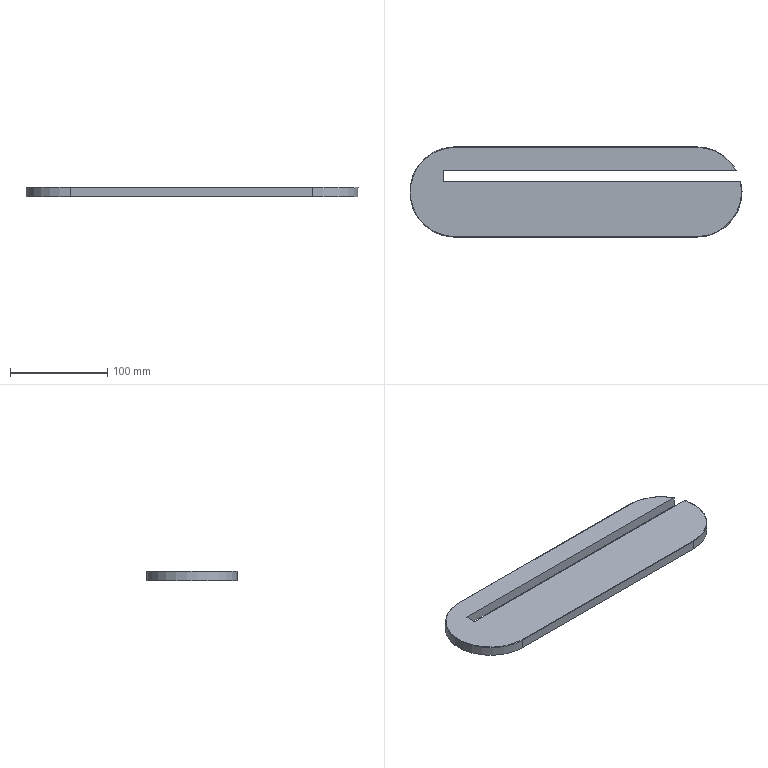Part | STEP file | DEWALT-DWE7492-B22 | 1 solid | 15 faces | box 342.3 x 93 x 10 mm | volume 265013 mm3 | plane 7 | cylinder 5 | torus 3 | commonest cylinder face diameters 93 x3 1 x2
STEP:
#1=CARTESIAN_POINT('',(0.,0.,0.));
#2=DIRECTION('',(0.,0.,1.));
#3=DIRECTION('',(1.,0.,0.));
#4=AXIS2_PLACEMENT_3D('',#1,#2,#3);
#5=CARTESIAN_POINT('',(-86.5,-1.8,30.));
#6=VERTEX_POINT('',#5);
#7=CARTESIAN_POINT('',(220.004,-1.8,30.));
#8=VERTEX_POINT('',#7);
#9=CARTESIAN_POINT('',(66.752,-1.8,30.));
#10=DIRECTION('',(1.,0.,0.));
#11=VECTOR('',#10,1.);
#12=LINE('',#9,#11);
#13=CARTESIAN_POINT('',(-86.51,-1.8,40.01));
#14=DIRECTION('',(0.,1.,0.));
#15=DIRECTION('',(1.,0.,0.));
#16=AXIS2_PLACEMENT_3D('',#13,#14,#15);
#17=PLANE('',#16);
#18=CARTESIAN_POINT('',(153.262,10.01));
#19=DIRECTION('',(1.,0.));
#20=VECTOR('',#19,1.);
#21=LINE('',#18,#20);
#22=(GEOMETRIC_REPRESENTATION_CONTEXT(2)PARAMETRIC_REPRESENTATION_CONTEXT()REPRESENTATION_CONTEXT('',''));
#23=DEFINITIONAL_REPRESENTATION('',(#21),#22);
#24=PCURVE('',#17,#23);
#25=CARTESIAN_POINT('',(-121.01,33.81,30.));
#26=DIRECTION('',(0.,0.,-1.));
#27=DIRECTION('',(1.,0.,0.));
#28=AXIS2_PLACEMENT_3D('',#25,#26,#27);
#29=PLANE('',#28);
#30=CARTESIAN_POINT('',(187.762,35.61));
#31=DIRECTION('',(1.,0.));
#32=VECTOR('',#31,1.);
#33=LINE('',#30,#32);
#34=(GEOMETRIC_REPRESENTATION_CONTEXT(2)PARAMETRIC_REPRESENTATION_CONTEXT()REPRESENTATION_CONTEXT('',''));
#35=DEFINITIONAL_REPRESENTATION('',(#33),#34);
#36=PCURVE('',#29,#35);
#37=SURFACE_CURVE('',#12,(#24,#36),.PCURVE_S1.);
#38=EDGE_CURVE('',#6,#8,#37,.T.);
#39=ORIENTED_EDGE('',*,*,#38,.F.);
#40=CARTESIAN_POINT('',(-86.5,-1.8,40.));
#41=VERTEX_POINT('',#40);
#42=CARTESIAN_POINT('',(-86.5,-1.8,35.));
#43=DIRECTION('',(0.,0.,-1.));
#44=VECTOR('',#43,1.);
#45=LINE('',#42,#44);
#46=CARTESIAN_POINT('',(0.01,5.01));
#47=DIRECTION('',(0.,1.));
#48=VECTOR('',#47,1.);
#49=LINE('',#46,#48);
#50=(GEOMETRIC_REPRESENTATION_CONTEXT(2)PARAMETRIC_REPRESENTATION_CONTEXT()REPRESENTATION_CONTEXT('',''));
#51=DEFINITIONAL_REPRESENTATION('',(#49),#50);
#52=PCURVE('',#17,#51);
#53=CARTESIAN_POINT('',(-86.5,9.61,40.01));
#54=DIRECTION('',(1.,0.,0.));
#55=DIRECTION('',(0.,-1.,0.));
#56=AXIS2_PLACEMENT_3D('',#53,#54,#55);
#57=PLANE('',#56);
#58=CARTESIAN_POINT('',(11.41,5.01));
#59=DIRECTION('',(0.,1.));
#60=VECTOR('',#59,1.);
#61=LINE('',#58,#60);
#62=(GEOMETRIC_REPRESENTATION_CONTEXT(2)PARAMETRIC_REPRESENTATION_CONTEXT()REPRESENTATION_CONTEXT('',''));
#63=DEFINITIONAL_REPRESENTATION('',(#61),#62);
#64=PCURVE('',#57,#63);
#65=SURFACE_CURVE('',#45,(#52,#64),.PCURVE_S1.);
#66=EDGE_CURVE('',#41,#6,#65,.T.);
#67=ORIENTED_EDGE('',*,*,#66,.F.);
#68=CARTESIAN_POINT('',(219.49,-1.8,40.));
#69=VERTEX_POINT('',#68);
#70=CARTESIAN_POINT('',(66.495,-1.8,40.));
#71=DIRECTION('',(-1.,0.,0.));
#72=VECTOR('',#71,1.);
#73=LINE('',#70,#72);
#74=CARTESIAN_POINT('',(153.005,0.01));
#75=DIRECTION('',(-1.,0.));
#76=VECTOR('',#75,1.);
#77=LINE('',#74,#76);
#78=(GEOMETRIC_REPRESENTATION_CONTEXT(2)PARAMETRIC_REPRESENTATION_CONTEXT()REPRESENTATION_CONTEXT('',''));
#79=DEFINITIONAL_REPRESENTATION('',(#77),#78);
#80=PCURVE('',#17,#79);
#81=CARTESIAN_POINT('',(224.799,33.31,40.));
#82=DIRECTION('',(0.,0.,1.));
#83=DIRECTION('',(-1.,0.,0.));
#84=AXIS2_PLACEMENT_3D('',#81,#82,#83);
#85=PLANE('',#84);
#86=CARTESIAN_POINT('',(158.304,35.11));
#87=DIRECTION('',(1.,0.));
#88=VECTOR('',#87,1.);
#89=LINE('',#86,#88);
#90=(GEOMETRIC_REPRESENTATION_CONTEXT(2)PARAMETRIC_REPRESENTATION_CONTEXT()REPRESENTATION_CONTEXT('',''));
#91=DEFINITIONAL_REPRESENTATION('',(#89),#90);
#92=PCURVE('',#85,#91);
#93=SURFACE_CURVE('',#73,(#80,#92),.PCURVE_S1.);
#94=EDGE_CURVE('',#69,#41,#93,.T.);
#95=ORIENTED_EDGE('',*,*,#94,.F.);
#96=CARTESIAN_POINT('',(220.004,-1.8,39.5));
#97=VERTEX_POINT('',#96);
#98=CARTESIAN_POINT('',(220.004,-1.8,39.5));
#99=CARTESIAN_POINT('',(220.004,-1.8,39.768));
#100=CARTESIAN_POINT('',(219.758,-1.8,40.));
#101=CARTESIAN_POINT('',(219.49,-1.8,40.));
#102=B_SPLINE_CURVE_WITH_KNOTS('',3,(#98,#99,#100,#101),.UNSPECIFIED.,.F.,.F.,(4,4),(0.,0.0007925),.PIECEWISE_BEZIER_KNOTS.);
#103=CARTESIAN_POINT('',(306.514,0.51));
#104=CARTESIAN_POINT('',(306.514,0.242));
#105=CARTESIAN_POINT('',(306.268,0.01));
#106=CARTESIAN_POINT('',(306.,0.01));
#107=B_SPLINE_CURVE_WITH_KNOTS('',3,(#103,#104,#105,#106),.UNSPECIFIED.,.F.,.F.,(4,4),(0.,0.0007925),.PIECEWISE_BEZIER_KNOTS.);
#108=(GEOMETRIC_REPRESENTATION_CONTEXT(2)PARAMETRIC_REPRESENTATION_CONTEXT()REPRESENTATION_CONTEXT('',''));
#109=DEFINITIONAL_REPRESENTATION('',(#107),#108);
#110=PCURVE('',#17,#109);
#111=CARTESIAN_POINT('',(174.8,-12.7,39.5));
#112=DIRECTION('',(0.,0.,1.));
#113=DIRECTION('',(0.,-1.,0.));
#114=AXIS2_PLACEMENT_3D('',#111,#112,#113);
#115=TOROIDAL_SURFACE('',#114,46.,0.5);
#116=CARTESIAN_POINT('',(1.807,0.));
#117=CARTESIAN_POINT('',(1.807,0.02436));
#118=CARTESIAN_POINT('',(1.807,0.0728));
#119=CARTESIAN_POINT('',(1.807,0.1448));
#120=CARTESIAN_POINT('',(1.807,0.2165));
#121=CARTESIAN_POINT('',(1.808,0.288));
#122=CARTESIAN_POINT('',(1.808,0.3594));
#123=CARTESIAN_POINT('',(1.808,0.4308));
#124=CARTESIAN_POINT('',(1.808,0.5024));
#125=CARTESIAN_POINT('',(1.808,0.5741));
#126=CARTESIAN_POINT('',(1.808,0.6458));
#127=CARTESIAN_POINT('',(1.808,0.7177));
#128=CARTESIAN_POINT('',(1.808,0.7896));
#129=CARTESIAN_POINT('',(1.808,0.8615));
#130=CARTESIAN_POINT('',(1.808,0.9332));
#131=CARTESIAN_POINT('',(1.809,1.005));
#132=CARTESIAN_POINT('',(1.809,1.076));
#133=CARTESIAN_POINT('',(1.809,1.147));
#134=CARTESIAN_POINT('',(1.809,1.218));
#135=CARTESIAN_POINT('',(1.809,1.289));
#136=CARTESIAN_POINT('',(1.809,1.359));
#137=CARTESIAN_POINT('',(1.81,1.43));
#138=CARTESIAN_POINT('',(1.81,1.5));
#139=CARTESIAN_POINT('',(1.81,1.547));
#140=CARTESIAN_POINT('',(1.81,1.571));
#141=B_SPLINE_CURVE_WITH_KNOTS('',3,(#116,#117,#118,#119,#120,#121,#122,#123,#124,#125,#126,#127,#128,#129,#130,#131,#132,#133,#134,#135,#136,#137,#138,#139,#140),.UNSPECIFIED.,.F.,.F.,(4,1,1,1,1,1,1,1,1,1,1,1,1,1,1,1,1,1,1,1,1,1,4),(0.,0.00003602,0.00007204,0.0001081,0.0001441,0.0001801,0.0002161,0.0002521,0.0002882,0.0003242,0.0003602,0.0003962,0.0004323,0.0004683,0.0005043,0.0005403,0.0005763,0.0006124,0.0006484,0.0006844,0.0007204,0.0007564,0.0007925),.QUASI_UNIFORM_KNOTS.);
#142=(GEOMETRIC_REPRESENTATION_CONTEXT(2)PARAMETRIC_REPRESENTATION_CONTEXT()REPRESENTATION_CONTEXT('',''));
#143=DEFINITIONAL_REPRESENTATION('',(#141),#142);
#144=PCURVE('',#115,#143);
#145=SURFACE_CURVE('',#102,(#110,#144),.PCURVE_S1.);
#146=EDGE_CURVE('',#97,#69,#145,.T.);
#147=ORIENTED_EDGE('',*,*,#146,.F.);
#148=CARTESIAN_POINT('',(220.004,-1.8,34.75));
#149=DIRECTION('',(0.,0.,1.));
#150=VECTOR('',#149,1.);
#151=LINE('',#148,#150);
#152=CARTESIAN_POINT('',(306.514,5.26));
#153=DIRECTION('',(0.,-1.));
#154=VECTOR('',#153,1.);
#155=LINE('',#152,#154);
#156=(GEOMETRIC_REPRESENTATION_CONTEXT(2)PARAMETRIC_REPRESENTATION_CONTEXT()REPRESENTATION_CONTEXT('',''));
#157=DEFINITIONAL_REPRESENTATION('',(#155),#156);
#158=PCURVE('',#17,#157);
#159=CARTESIAN_POINT('',(174.8,-12.7,30.));
#160=DIRECTION('',(0.,0.,1.));
#161=DIRECTION('',(1.,0.,0.));
#162=AXIS2_PLACEMENT_3D('',#159,#160,#161);
#163=CYLINDRICAL_SURFACE('',#162,46.5);
#164=CARTESIAN_POINT('',(6.52,4.75));
#165=DIRECTION('',(0.,1.));
#166=VECTOR('',#165,1.);
#167=LINE('',#164,#166);
#168=(GEOMETRIC_REPRESENTATION_CONTEXT(2)PARAMETRIC_REPRESENTATION_CONTEXT()REPRESENTATION_CONTEXT('',''));
#169=DEFINITIONAL_REPRESENTATION('',(#167),#168);
#170=PCURVE('',#163,#169);
#171=SURFACE_CURVE('',#151,(#158,#170),.PCURVE_S1.);
#172=EDGE_CURVE('',#8,#97,#171,.T.);
#173=ORIENTED_EDGE('',*,*,#172,.F.);
#174=EDGE_LOOP('',(#39,#67,#95,#147,#173));
#175=FACE_BOUND('',#174,.T.);
#176=ADVANCED_FACE('',(#175),#17,.T.);
#177=CARTESIAN_POINT('',(215.604,9.6,30.));
#178=VERTEX_POINT('',#177);
#179=CARTESIAN_POINT('',(-86.5,9.6,30.));
#180=VERTEX_POINT('',#179);
#181=CARTESIAN_POINT('',(64.552,9.6,30.));
#182=DIRECTION('',(-1.,0.,0.));
#183=VECTOR('',#182,1.);
#184=LINE('',#181,#183);
#185=CARTESIAN_POINT('',(215.614,9.6,40.01));
#186=DIRECTION('',(0.,-1.,0.));
#187=DIRECTION('',(-1.,0.,0.));
#188=AXIS2_PLACEMENT_3D('',#185,#186,#187);
#189=PLANE('',#188);
#190=CARTESIAN_POINT('',(151.062,10.01));
#191=DIRECTION('',(1.,0.));
#192=VECTOR('',#191,1.);
#193=LINE('',#190,#192);
#194=(GEOMETRIC_REPRESENTATION_CONTEXT(2)PARAMETRIC_REPRESENTATION_CONTEXT()REPRESENTATION_CONTEXT('',''));
#195=DEFINITIONAL_REPRESENTATION('',(#193),#194);
#196=PCURVE('',#189,#195);
#197=CARTESIAN_POINT('',(185.562,24.21));
#198=DIRECTION('',(-1.,0.));
#199=VECTOR('',#198,1.);
#200=LINE('',#197,#199);
#201=(GEOMETRIC_REPRESENTATION_CONTEXT(2)PARAMETRIC_REPRESENTATION_CONTEXT()REPRESENTATION_CONTEXT('',''));
#202=DEFINITIONAL_REPRESENTATION('',(#200),#201);
#203=PCURVE('',#29,#202);
#204=SURFACE_CURVE('',#184,(#196,#203),.PCURVE_S1.);
#205=EDGE_CURVE('',#178,#180,#204,.T.);
#206=ORIENTED_EDGE('',*,*,#205,.F.);
#207=CARTESIAN_POINT('',(215.604,9.6,39.5));
#208=VERTEX_POINT('',#207);
#209=CARTESIAN_POINT('',(215.604,9.6,34.75));
#210=DIRECTION('',(0.,0.,-1.));
#211=VECTOR('',#210,1.);
#212=LINE('',#209,#211);
#213=CARTESIAN_POINT('',(0.01,5.26));
#214=DIRECTION('',(0.,1.));
#215=VECTOR('',#214,1.);
#216=LINE('',#213,#215);
#217=(GEOMETRIC_REPRESENTATION_CONTEXT(2)PARAMETRIC_REPRESENTATION_CONTEXT()REPRESENTATION_CONTEXT('',''));
#218=DEFINITIONAL_REPRESENTATION('',(#216),#217);
#219=PCURVE('',#189,#218);
#220=CARTESIAN_POINT('',(174.8,-12.7,30.));
#221=DIRECTION('',(0.,0.,1.));
#222=DIRECTION('',(0.,-1.,0.));
#223=AXIS2_PLACEMENT_3D('',#220,#221,#222);
#224=CYLINDRICAL_SURFACE('',#223,46.5);
#225=CARTESIAN_POINT('',(2.071,4.75));
#226=DIRECTION('',(0.,-1.));
#227=VECTOR('',#226,1.);
#228=LINE('',#225,#227);
#229=(GEOMETRIC_REPRESENTATION_CONTEXT(2)PARAMETRIC_REPRESENTATION_CONTEXT()REPRESENTATION_CONTEXT('',''));
#230=DEFINITIONAL_REPRESENTATION('',(#228),#229);
#231=PCURVE('',#224,#230);
#232=SURFACE_CURVE('',#212,(#219,#231),.PCURVE_S1.);
#233=EDGE_CURVE('',#208,#178,#232,.T.);
#234=ORIENTED_EDGE('',*,*,#233,.F.);
#235=CARTESIAN_POINT('',(215.033,9.6,40.));
#236=VERTEX_POINT('',#235);
#237=CARTESIAN_POINT('',(215.033,9.6,40.));
#238=CARTESIAN_POINT('',(215.316,9.6,40.));
#239=CARTESIAN_POINT('',(215.604,9.6,39.784));
#240=CARTESIAN_POINT('',(215.604,9.6,39.5));
#241=B_SPLINE_CURVE_WITH_KNOTS('',3,(#237,#238,#239,#240),.UNSPECIFIED.,.F.,.F.,(4,4),(0.,0.0008376),.PIECEWISE_BEZIER_KNOTS.);
#242=CARTESIAN_POINT('',(0.5807,0.01));
#243=CARTESIAN_POINT('',(0.2976,0.01));
#244=CARTESIAN_POINT('',(0.01,0.2255));
#245=CARTESIAN_POINT('',(0.01,0.51));
#246=B_SPLINE_CURVE_WITH_KNOTS('',3,(#242,#243,#244,#245),.UNSPECIFIED.,.F.,.F.,(4,4),(0.,0.0008376),.PIECEWISE_BEZIER_KNOTS.);
#247=(GEOMETRIC_REPRESENTATION_CONTEXT(2)PARAMETRIC_REPRESENTATION_CONTEXT()REPRESENTATION_CONTEXT('',''));
#248=DEFINITIONAL_REPRESENTATION('',(#246),#247);
#249=PCURVE('',#189,#248);
#250=CARTESIAN_POINT('',(174.8,-12.7,39.5));
#251=DIRECTION('',(0.,0.,1.));
#252=DIRECTION('',(1.,0.,0.));
#253=AXIS2_PLACEMENT_3D('',#250,#251,#252);
#254=TOROIDAL_SURFACE('',#253,46.,0.5);
#255=CARTESIAN_POINT('',(0.5061,1.571));
#256=CARTESIAN_POINT('',(0.506,1.548));
#257=CARTESIAN_POINT('',(0.5057,1.503));
#258=CARTESIAN_POINT('',(0.5053,1.435));
#259=CARTESIAN_POINT('',(0.5049,1.367));
#260=CARTESIAN_POINT('',(0.5045,1.298));
#261=CARTESIAN_POINT('',(0.5041,1.229));
#262=CARTESIAN_POINT('',(0.5037,1.16));
#263=CARTESIAN_POINT('',(0.5034,1.089));
#264=CARTESIAN_POINT('',(0.503,1.019));
#265=CARTESIAN_POINT('',(0.5027,0.9479));
#266=CARTESIAN_POINT('',(0.5023,0.8767));
#267=CARTESIAN_POINT('',(0.502,0.8052));
#268=CARTESIAN_POINT('',(0.5017,0.7336));
#269=CARTESIAN_POINT('',(0.5014,0.6618));
#270=CARTESIAN_POINT('',(0.5012,0.5899));
#271=CARTESIAN_POINT('',(0.501,0.5178));
#272=CARTESIAN_POINT('',(0.5008,0.4456));
#273=CARTESIAN_POINT('',(0.5006,0.3731));
#274=CARTESIAN_POINT('',(0.5004,0.3002));
#275=CARTESIAN_POINT('',(0.5003,0.2267));
#276=CARTESIAN_POINT('',(0.5002,0.1524));
#277=CARTESIAN_POINT('',(0.5002,0.07701));
#278=CARTESIAN_POINT('',(0.5002,0.02586));
#279=CARTESIAN_POINT('',(0.5002,0.));
#280=B_SPLINE_CURVE_WITH_KNOTS('',3,(#255,#256,#257,#258,#259,#260,#261,#262,#263,#264,#265,#266,#267,#268,#269,#270,#271,#272,#273,#274,#275,#276,#277,#278,#279),.UNSPECIFIED.,.F.,.F.,(4,1,1,1,1,1,1,1,1,1,1,1,1,1,1,1,1,1,1,1,1,1,4),(0.,0.00003807,0.00007615,0.0001142,0.0001523,0.0001904,0.0002284,0.0002665,0.0003046,0.0003427,0.0003807,0.0004188,0.0004569,0.000495,0.000533,0.0005711,0.0006092,0.0006473,0.0006853,0.0007234,0.0007615,0.0007996,0.0008376),.QUASI_UNIFORM_KNOTS.);
#281=(GEOMETRIC_REPRESENTATION_CONTEXT(2)PARAMETRIC_REPRESENTATION_CONTEXT()REPRESENTATION_CONTEXT('',''));
#282=DEFINITIONAL_REPRESENTATION('',(#280),#281);
#283=PCURVE('',#254,#282);
#284=SURFACE_CURVE('',#241,(#249,#283),.PCURVE_S1.);
#285=EDGE_CURVE('',#236,#208,#284,.T.);
#286=ORIENTED_EDGE('',*,*,#285,.F.);
#287=CARTESIAN_POINT('',(-86.5,9.6,40.));
#288=VERTEX_POINT('',#287);
#289=CARTESIAN_POINT('',(64.267,9.6,40.));
#290=DIRECTION('',(1.,0.,0.));
#291=VECTOR('',#290,1.);
#292=LINE('',#289,#291);
#293=CARTESIAN_POINT('',(151.347,0.01));
#294=DIRECTION('',(-1.,0.));
#295=VECTOR('',#294,1.);
#296=LINE('',#293,#295);
#297=(GEOMETRIC_REPRESENTATION_CONTEXT(2)PARAMETRIC_REPRESENTATION_CONTEXT()REPRESENTATION_CONTEXT('',''));
#298=DEFINITIONAL_REPRESENTATION('',(#296),#297);
#299=PCURVE('',#189,#298);
#300=CARTESIAN_POINT('',(160.532,23.71));
#301=DIRECTION('',(-1.,0.));
#302=VECTOR('',#301,1.);
#303=LINE('',#300,#302);
#304=(GEOMETRIC_REPRESENTATION_CONTEXT(2)PARAMETRIC_REPRESENTATION_CONTEXT()REPRESENTATION_CONTEXT('',''));
#305=DEFINITIONAL_REPRESENTATION('',(#303),#304);
#306=PCURVE('',#85,#305);
#307=SURFACE_CURVE('',#292,(#299,#306),.PCURVE_S1.);
#308=EDGE_CURVE('',#288,#236,#307,.T.);
#309=ORIENTED_EDGE('',*,*,#308,.F.);
#310=CARTESIAN_POINT('',(-86.5,9.6,35.));
#311=DIRECTION('',(0.,0.,-1.));
#312=VECTOR('',#311,1.);
#313=LINE('',#310,#312);
#314=CARTESIAN_POINT('',(302.114,5.01));
#315=DIRECTION('',(0.,1.));
#316=VECTOR('',#315,1.);
#317=LINE('',#314,#316);
#318=(GEOMETRIC_REPRESENTATION_CONTEXT(2)PARAMETRIC_REPRESENTATION_CONTEXT()REPRESENTATION_CONTEXT('',''));
#319=DEFINITIONAL_REPRESENTATION('',(#317),#318);
#320=PCURVE('',#189,#319);
#321=CARTESIAN_POINT('',(0.01,5.01));
#322=DIRECTION('',(0.,1.));
#323=VECTOR('',#322,1.);
#324=LINE('',#321,#323);
#325=(GEOMETRIC_REPRESENTATION_CONTEXT(2)PARAMETRIC_REPRESENTATION_CONTEXT()REPRESENTATION_CONTEXT('',''));
#326=DEFINITIONAL_REPRESENTATION('',(#324),#325);
#327=PCURVE('',#57,#326);
#328=SURFACE_CURVE('',#313,(#320,#327),.PCURVE_S1.);
#329=EDGE_CURVE('',#288,#180,#328,.T.);
#330=ORIENTED_EDGE('',*,*,#329,.T.);
#331=EDGE_LOOP('',(#206,#234,#286,#309,#330));
#332=FACE_BOUND('',#331,.T.);
#333=ADVANCED_FACE('',(#332),#189,.T.);
#334=CARTESIAN_POINT('',(-86.5,3.9,30.));
#335=DIRECTION('',(0.,-1.,0.));
#336=VECTOR('',#335,1.);
#337=LINE('',#334,#336);
#338=CARTESIAN_POINT('',(5.71,10.01));
#339=DIRECTION('',(1.,0.));
#340=VECTOR('',#339,1.);
#341=LINE('',#338,#340);
#342=(GEOMETRIC_REPRESENTATION_CONTEXT(2)PARAMETRIC_REPRESENTATION_CONTEXT()REPRESENTATION_CONTEXT('',''));
#343=DEFINITIONAL_REPRESENTATION('',(#341),#342);
#344=PCURVE('',#57,#343);
#345=CARTESIAN_POINT('',(34.51,29.91));
#346=DIRECTION('',(0.,1.));
#347=VECTOR('',#346,1.);
#348=LINE('',#345,#347);
#349=(GEOMETRIC_REPRESENTATION_CONTEXT(2)PARAMETRIC_REPRESENTATION_CONTEXT()REPRESENTATION_CONTEXT('',''));
#350=DEFINITIONAL_REPRESENTATION('',(#348),#349);
#351=PCURVE('',#29,#350);
#352=SURFACE_CURVE('',#337,(#344,#351),.PCURVE_S1.);
#353=EDGE_CURVE('',#180,#6,#352,.T.);
#354=ORIENTED_EDGE('',*,*,#353,.F.);
#355=ORIENTED_EDGE('',*,*,#329,.F.);
#356=CARTESIAN_POINT('',(-86.5,3.9,40.));
#357=DIRECTION('',(0.,1.,0.));
#358=VECTOR('',#357,1.);
#359=LINE('',#356,#358);
#360=CARTESIAN_POINT('',(5.71,0.01));
#361=DIRECTION('',(-1.,0.));
#362=VECTOR('',#361,1.);
#363=LINE('',#360,#362);
#364=(GEOMETRIC_REPRESENTATION_CONTEXT(2)PARAMETRIC_REPRESENTATION_CONTEXT()REPRESENTATION_CONTEXT('',''));
#365=DEFINITIONAL_REPRESENTATION('',(#363),#364);
#366=PCURVE('',#57,#365);
#367=CARTESIAN_POINT('',(311.299,29.41));
#368=DIRECTION('',(0.,-1.));
#369=VECTOR('',#368,1.);
#370=LINE('',#367,#369);
#371=(GEOMETRIC_REPRESENTATION_CONTEXT(2)PARAMETRIC_REPRESENTATION_CONTEXT()REPRESENTATION_CONTEXT('',''));
#372=DEFINITIONAL_REPRESENTATION('',(#370),#371);
#373=PCURVE('',#85,#372);
#374=SURFACE_CURVE('',#359,(#366,#373),.PCURVE_S1.);
#375=EDGE_CURVE('',#41,#288,#374,.T.);
#376=ORIENTED_EDGE('',*,*,#375,.F.);
#377=ORIENTED_EDGE('',*,*,#66,.T.);
#378=EDGE_LOOP('',(#354,#355,#376,#377));
#379=FACE_BOUND('',#378,.T.);
#380=ADVANCED_FACE('',(#379),#57,.T.);
#381=ORIENTED_EDGE('',*,*,#94,.T.);
#382=ORIENTED_EDGE('',*,*,#375,.T.);
#383=ORIENTED_EDGE('',*,*,#308,.T.);
#384=CARTESIAN_POINT('',(174.8,33.3,40.));
#385=VERTEX_POINT('',#384);
#386=CARTESIAN_POINT('',(174.8,-12.7,40.));
#387=DIRECTION('',(0.,0.,-1.));
#388=DIRECTION('',(0.,1.,0.));
#389=AXIS2_PLACEMENT_3D('',#386,#387,#388);
#390=CIRCLE('',#389,46.);
#391=CARTESIAN_POINT('',(49.999,0.01));
#392=CARTESIAN_POINT('',(-29.675,0.01));
#393=CARTESIAN_POINT('',(10.162,69.01));
#394=CARTESIAN_POINT('',(49.999,138.01));
#395=CARTESIAN_POINT('',(89.836,69.01));
#396=CARTESIAN_POINT('',(129.673,0.01));
#397=CARTESIAN_POINT('',(49.999,0.01));
#398=(BOUNDED_CURVE()B_SPLINE_CURVE(2,(#391,#392,#393,#394,#395,#396,#397),.UNSPECIFIED.,.T.,.F.)B_SPLINE_CURVE_WITH_KNOTS((1,2,2,2,2,1),(-2.094,0.,2.094,4.189,6.283,8.378),.UNSPECIFIED.)CURVE()GEOMETRIC_REPRESENTATION_ITEM()RATIONAL_B_SPLINE_CURVE((1.,0.5,1.,0.5,1.,0.5,1.))REPRESENTATION_ITEM(''));
#399=(GEOMETRIC_REPRESENTATION_CONTEXT(2)PARAMETRIC_REPRESENTATION_CONTEXT()REPRESENTATION_CONTEXT('',''));
#400=DEFINITIONAL_REPRESENTATION('',(#398),#399);
#401=PCURVE('',#85,#400);
#402=CARTESIAN_POINT('',(1.571,1.571));
#403=DIRECTION('',(-1.,0.));
#404=VECTOR('',#403,1.);
#405=LINE('',#402,#404);
#406=(GEOMETRIC_REPRESENTATION_CONTEXT(2)PARAMETRIC_REPRESENTATION_CONTEXT()REPRESENTATION_CONTEXT('',''));
#407=DEFINITIONAL_REPRESENTATION('',(#405),#406);
#408=PCURVE('',#254,#407);
#409=SURFACE_CURVE('',#390,(#401,#408),.PCURVE_S1.);
#410=EDGE_CURVE('',#385,#236,#409,.T.);
#411=ORIENTED_EDGE('',*,*,#410,.F.);
#412=CARTESIAN_POINT('',(-74.5,33.3,40.));
#413=VERTEX_POINT('',#412);
#414=CARTESIAN_POINT('',(50.15,33.3,40.));
#415=DIRECTION('',(1.,0.,0.));
#416=VECTOR('',#415,1.);
#417=LINE('',#414,#416);
#418=CARTESIAN_POINT('',(174.649,0.01));
#419=DIRECTION('',(-1.,0.));
#420=VECTOR('',#419,1.);
#421=LINE('',#418,#420);
#422=(GEOMETRIC_REPRESENTATION_CONTEXT(2)PARAMETRIC_REPRESENTATION_CONTEXT()REPRESENTATION_CONTEXT('',''));
#423=DEFINITIONAL_REPRESENTATION('',(#421),#422);
#424=PCURVE('',#85,#423);
#425=CARTESIAN_POINT('',(-74.5,33.3,39.5));
#426=DIRECTION('',(1.,0.,0.));
#427=DIRECTION('',(0.,1.,0.));
#428=AXIS2_PLACEMENT_3D('',#425,#426,#427);
#429=CYLINDRICAL_SURFACE('',#428,0.5);
#430=CARTESIAN_POINT('',(1.571,124.65));
#431=DIRECTION('',(0.,1.));
#432=VECTOR('',#431,1.);
#433=LINE('',#430,#432);
#434=(GEOMETRIC_REPRESENTATION_CONTEXT(2)PARAMETRIC_REPRESENTATION_CONTEXT()REPRESENTATION_CONTEXT('',''));
#435=DEFINITIONAL_REPRESENTATION('',(#433),#434);
#436=PCURVE('',#429,#435);
#437=SURFACE_CURVE('',#417,(#424,#436),.PCURVE_S1.);
#438=EDGE_CURVE('',#413,#385,#437,.T.);
#439=ORIENTED_EDGE('',*,*,#438,.F.);
#440=CARTESIAN_POINT('',(-74.5,-58.7,40.));
#441=VERTEX_POINT('',#440);
#442=CARTESIAN_POINT('',(-74.5,-12.7,40.));
#443=DIRECTION('',(0.,0.,-1.));
#444=DIRECTION('',(0.,-1.,0.));
#445=AXIS2_PLACEMENT_3D('',#442,#443,#444);
#446=CIRCLE('',#445,46.);
#447=CARTESIAN_POINT('',(299.299,92.01));
#448=CARTESIAN_POINT('',(378.973,92.01));
#449=CARTESIAN_POINT('',(339.136,23.01));
#450=CARTESIAN_POINT('',(299.299,-45.99));
#451=CARTESIAN_POINT('',(259.462,23.01));
#452=CARTESIAN_POINT('',(219.625,92.01));
#453=CARTESIAN_POINT('',(299.299,92.01));
#454=(BOUNDED_CURVE()B_SPLINE_CURVE(2,(#447,#448,#449,#450,#451,#452,#453),.UNSPECIFIED.,.T.,.F.)B_SPLINE_CURVE_WITH_KNOTS((1,2,2,2,2,1),(-2.094,0.,2.094,4.189,6.283,8.378),.UNSPECIFIED.)CURVE()GEOMETRIC_REPRESENTATION_ITEM()RATIONAL_B_SPLINE_CURVE((1.,0.5,1.,0.5,1.,0.5,1.))REPRESENTATION_ITEM(''));
#455=(GEOMETRIC_REPRESENTATION_CONTEXT(2)PARAMETRIC_REPRESENTATION_CONTEXT()REPRESENTATION_CONTEXT('',''));
#456=DEFINITIONAL_REPRESENTATION('',(#454),#455);
#457=PCURVE('',#85,#456);
#458=CARTESIAN_POINT('',(-74.5,-12.7,39.5));
#459=DIRECTION('',(0.,0.,1.));
#460=DIRECTION('',(1.,0.,0.));
#461=AXIS2_PLACEMENT_3D('',#458,#459,#460);
#462=TOROIDAL_SURFACE('',#461,46.,0.5);
#463=CARTESIAN_POINT('',(4.712,1.571));
#464=DIRECTION('',(-1.,0.));
#465=VECTOR('',#464,1.);
#466=LINE('',#463,#465);
#467=(GEOMETRIC_REPRESENTATION_CONTEXT(2)PARAMETRIC_REPRESENTATION_CONTEXT()REPRESENTATION_CONTEXT('',''));
#468=DEFINITIONAL_REPRESENTATION('',(#466),#467);
#469=PCURVE('',#462,#468);
#470=SURFACE_CURVE('',#446,(#457,#469),.PCURVE_S1.);
#471=EDGE_CURVE('',#441,#413,#470,.T.);
#472=ORIENTED_EDGE('',*,*,#471,.F.);
#473=CARTESIAN_POINT('',(174.8,-58.7,40.));
#474=VERTEX_POINT('',#473);
#475=CARTESIAN_POINT('',(50.15,-58.7,40.));
#476=DIRECTION('',(-1.,0.,0.));
#477=VECTOR('',#476,1.);
#478=LINE('',#475,#477);
#479=CARTESIAN_POINT('',(174.649,92.01));
#480=DIRECTION('',(1.,0.));
#481=VECTOR('',#480,1.);
#482=LINE('',#479,#481);
#483=(GEOMETRIC_REPRESENTATION_CONTEXT(2)PARAMETRIC_REPRESENTATION_CONTEXT()REPRESENTATION_CONTEXT('',''));
#484=DEFINITIONAL_REPRESENTATION('',(#482),#483);
#485=PCURVE('',#85,#484);
#486=CARTESIAN_POINT('',(174.8,-58.7,39.5));
#487=DIRECTION('',(-1.,0.,0.));
#488=DIRECTION('',(0.,0.,1.));
#489=AXIS2_PLACEMENT_3D('',#486,#487,#488);
#490=CYLINDRICAL_SURFACE('',#489,0.5);
#491=CARTESIAN_POINT('',(6.283,124.65));
#492=DIRECTION('',(0.,1.));
#493=VECTOR('',#492,1.);
#494=LINE('',#491,#493);
#495=(GEOMETRIC_REPRESENTATION_CONTEXT(2)PARAMETRIC_REPRESENTATION_CONTEXT()REPRESENTATION_CONTEXT('',''));
#496=DEFINITIONAL_REPRESENTATION('',(#494),#495);
#497=PCURVE('',#490,#496);
#498=SURFACE_CURVE('',#478,(#485,#497),.PCURVE_S1.);
#499=EDGE_CURVE('',#474,#441,#498,.T.);
#500=ORIENTED_EDGE('',*,*,#499,.F.);
#501=CARTESIAN_POINT('',(174.8,-12.7,40.));
#502=DIRECTION('',(0.,0.,-1.));
#503=DIRECTION('',(0.9715,0.237,0.));
#504=AXIS2_PLACEMENT_3D('',#501,#502,#503);
#505=CIRCLE('',#504,46.);
#506=CARTESIAN_POINT('',(5.309,35.11));
#507=CARTESIAN_POINT('',(-13.57,112.515));
#508=CARTESIAN_POINT('',(62.904,90.163));
#509=CARTESIAN_POINT('',(139.379,67.81));
#510=CARTESIAN_POINT('',(81.784,12.757));
#511=CARTESIAN_POINT('',(24.188,-42.295));
#512=CARTESIAN_POINT('',(5.309,35.11));
#513=(BOUNDED_CURVE()B_SPLINE_CURVE(2,(#506,#507,#508,#509,#510,#511,#512),.UNSPECIFIED.,.T.,.F.)B_SPLINE_CURVE_WITH_KNOTS((1,2,2,2,2,1),(-2.094,0.,2.094,4.189,6.283,8.378),.UNSPECIFIED.)CURVE()GEOMETRIC_REPRESENTATION_ITEM()RATIONAL_B_SPLINE_CURVE((1.,0.5,1.,0.5,1.,0.5,1.))REPRESENTATION_ITEM(''));
#514=(GEOMETRIC_REPRESENTATION_CONTEXT(2)PARAMETRIC_REPRESENTATION_CONTEXT()REPRESENTATION_CONTEXT('',''));
#515=DEFINITIONAL_REPRESENTATION('',(#513),#514);
#516=PCURVE('',#85,#515);
#517=CARTESIAN_POINT('',(1.81,1.571));
#518=DIRECTION('',(-1.,0.));
#519=VECTOR('',#518,1.);
#520=LINE('',#517,#519);
#521=(GEOMETRIC_REPRESENTATION_CONTEXT(2)PARAMETRIC_REPRESENTATION_CONTEXT()REPRESENTATION_CONTEXT('',''));
#522=DEFINITIONAL_REPRESENTATION('',(#520),#521);
#523=PCURVE('',#115,#522);
#524=SURFACE_CURVE('',#505,(#516,#523),.PCURVE_S1.);
#525=EDGE_CURVE('',#69,#474,#524,.T.);
#526=ORIENTED_EDGE('',*,*,#525,.F.);
#527=EDGE_LOOP('',(#381,#382,#383,#411,#439,#472,#500,#526));
#528=FACE_BOUND('',#527,.T.);
#529=ADVANCED_FACE('',(#528),#85,.T.);
#530=ORIENTED_EDGE('',*,*,#233,.T.);
#531=CARTESIAN_POINT('',(174.8,33.8,30.));
#532=VERTEX_POINT('',#531);
#533=CARTESIAN_POINT('',(174.8,-12.7,30.));
#534=DIRECTION('',(0.,0.,-1.));
#535=DIRECTION('',(0.,1.,0.));
#536=AXIS2_PLACEMENT_3D('',#533,#534,#535);
#537=CIRCLE('',#536,46.5);
#538=CARTESIAN_POINT('',(3.142,0.));
#539=DIRECTION('',(-1.,0.));
#540=VECTOR('',#539,1.);
#541=LINE('',#538,#540);
#542=(GEOMETRIC_REPRESENTATION_CONTEXT(2)PARAMETRIC_REPRESENTATION_CONTEXT()REPRESENTATION_CONTEXT('',''));
#543=DEFINITIONAL_REPRESENTATION('',(#541),#542);
#544=PCURVE('',#224,#543);
#545=CARTESIAN_POINT('',(295.81,46.51));
#546=DIRECTION('',(0.,-1.));
#547=AXIS2_PLACEMENT_2D('',#545,#546);
#548=CIRCLE('',#547,46.5);
#549=(GEOMETRIC_REPRESENTATION_CONTEXT(2)PARAMETRIC_REPRESENTATION_CONTEXT()REPRESENTATION_CONTEXT('',''));
#550=DEFINITIONAL_REPRESENTATION('',(#548),#549);
#551=PCURVE('',#29,#550);
#552=SURFACE_CURVE('',#537,(#544,#551),.PCURVE_S1.);
#553=EDGE_CURVE('',#532,#178,#552,.T.);
#554=ORIENTED_EDGE('',*,*,#553,.F.);
#555=CARTESIAN_POINT('',(174.8,33.8,39.5));
#556=VERTEX_POINT('',#555);
#557=CARTESIAN_POINT('',(174.8,33.8,34.75));
#558=DIRECTION('',(0.,0.,-1.));
#559=VECTOR('',#558,1.);
#560=LINE('',#557,#559);
#561=CARTESIAN_POINT('',(3.142,4.75));
#562=DIRECTION('',(0.,-1.));
#563=VECTOR('',#562,1.);
#564=LINE('',#561,#563);
#565=(GEOMETRIC_REPRESENTATION_CONTEXT(2)PARAMETRIC_REPRESENTATION_CONTEXT()REPRESENTATION_CONTEXT('',''));
#566=DEFINITIONAL_REPRESENTATION('',(#564),#565);
#567=PCURVE('',#224,#566);
#568=CARTESIAN_POINT('',(-74.51,33.8,39.51));
#569=DIRECTION('',(0.,1.,0.));
#570=DIRECTION('',(1.,0.,0.));
#571=AXIS2_PLACEMENT_3D('',#568,#569,#570);
#572=PLANE('',#571);
#573=CARTESIAN_POINT('',(249.31,4.76));
#574=DIRECTION('',(0.,1.));
#575=VECTOR('',#574,1.);
#576=LINE('',#573,#575);
#577=(GEOMETRIC_REPRESENTATION_CONTEXT(2)PARAMETRIC_REPRESENTATION_CONTEXT()REPRESENTATION_CONTEXT('',''));
#578=DEFINITIONAL_REPRESENTATION('',(#576),#577);
#579=PCURVE('',#572,#578);
#580=SURFACE_CURVE('',#560,(#567,#579),.PCURVE_S1.);
#581=EDGE_CURVE('',#556,#532,#580,.T.);
#582=ORIENTED_EDGE('',*,*,#581,.F.);
#583=CARTESIAN_POINT('',(174.8,-12.7,39.5));
#584=DIRECTION('',(0.,0.,1.));
#585=DIRECTION('',(0.8775,0.4796,0.));
#586=AXIS2_PLACEMENT_3D('',#583,#584,#585);
#587=CIRCLE('',#586,46.5);
#588=CARTESIAN_POINT('',(2.071,9.5));
#589=DIRECTION('',(1.,0.));
#590=VECTOR('',#589,1.);
#591=LINE('',#588,#590);
#592=(GEOMETRIC_REPRESENTATION_CONTEXT(2)PARAMETRIC_REPRESENTATION_CONTEXT()REPRESENTATION_CONTEXT('',''));
#593=DEFINITIONAL_REPRESENTATION('',(#591),#592);
#594=PCURVE('',#224,#593);
#595=CARTESIAN_POINT('',(0.5002,0.));
#596=DIRECTION('',(1.,0.));
#597=VECTOR('',#596,1.);
#598=LINE('',#595,#597);
#599=(GEOMETRIC_REPRESENTATION_CONTEXT(2)PARAMETRIC_REPRESENTATION_CONTEXT()REPRESENTATION_CONTEXT('',''));
#600=DEFINITIONAL_REPRESENTATION('',(#598),#599);
#601=PCURVE('',#254,#600);
#602=SURFACE_CURVE('',#587,(#594,#601),.PCURVE_S1.);
#603=EDGE_CURVE('',#208,#556,#602,.T.);
#604=ORIENTED_EDGE('',*,*,#603,.F.);
#605=EDGE_LOOP('',(#530,#554,#582,#604));
#606=FACE_BOUND('',#605,.T.);
#607=ADVANCED_FACE('',(#606),#224,.T.);
#608=ORIENTED_EDGE('',*,*,#172,.T.);
#609=CARTESIAN_POINT('',(174.8,-59.2,39.5));
#610=VERTEX_POINT('',#609);
#611=CARTESIAN_POINT('',(174.8,-12.7,39.5));
#612=DIRECTION('',(0.,0.,1.));
#613=DIRECTION('',(0.,-1.,0.));
#614=AXIS2_PLACEMENT_3D('',#611,#612,#613);
#615=CIRCLE('',#614,46.5);
#616=CARTESIAN_POINT('',(4.712,9.5));
#617=DIRECTION('',(1.,0.));
#618=VECTOR('',#617,1.);
#619=LINE('',#616,#618);
#620=(GEOMETRIC_REPRESENTATION_CONTEXT(2)PARAMETRIC_REPRESENTATION_CONTEXT()REPRESENTATION_CONTEXT('',''));
#621=DEFINITIONAL_REPRESENTATION('',(#619),#620);
#622=PCURVE('',#163,#621);
#623=CARTESIAN_POINT('',(0.,0.));
#624=DIRECTION('',(1.,0.));
#625=VECTOR('',#624,1.);
#626=LINE('',#623,#625);
#627=(GEOMETRIC_REPRESENTATION_CONTEXT(2)PARAMETRIC_REPRESENTATION_CONTEXT()REPRESENTATION_CONTEXT('',''));
#628=DEFINITIONAL_REPRESENTATION('',(#626),#627);
#629=PCURVE('',#115,#628);
#630=SURFACE_CURVE('',#615,(#622,#629),.PCURVE_S1.);
#631=EDGE_CURVE('',#610,#97,#630,.T.);
#632=ORIENTED_EDGE('',*,*,#631,.F.);
#633=CARTESIAN_POINT('',(174.8,-59.2,30.));
#634=VERTEX_POINT('',#633);
#635=CARTESIAN_POINT('',(174.8,-59.2,34.75));
#636=DIRECTION('',(0.,0.,-1.));
#637=VECTOR('',#636,1.);
#638=LINE('',#635,#637);
#639=CARTESIAN_POINT('',(4.712,4.75));
#640=DIRECTION('',(0.,-1.));
#641=VECTOR('',#640,1.);
#642=LINE('',#639,#641);
#643=(GEOMETRIC_REPRESENTATION_CONTEXT(2)PARAMETRIC_REPRESENTATION_CONTEXT()REPRESENTATION_CONTEXT('',''));
#644=DEFINITIONAL_REPRESENTATION('',(#642),#643);
#645=PCURVE('',#163,#644);
#646=CARTESIAN_POINT('',(174.81,-59.2,39.51));
#647=DIRECTION('',(0.,-1.,0.));
#648=DIRECTION('',(-1.,0.,0.));
#649=AXIS2_PLACEMENT_3D('',#646,#647,#648);
#650=PLANE('',#649);
#651=CARTESIAN_POINT('',(0.01,4.76));
#652=DIRECTION('',(0.,1.));
#653=VECTOR('',#652,1.);
#654=LINE('',#651,#653);
#655=(GEOMETRIC_REPRESENTATION_CONTEXT(2)PARAMETRIC_REPRESENTATION_CONTEXT()REPRESENTATION_CONTEXT('',''));
#656=DEFINITIONAL_REPRESENTATION('',(#654),#655);
#657=PCURVE('',#650,#656);
#658=SURFACE_CURVE('',#638,(#645,#657),.PCURVE_S1.);
#659=EDGE_CURVE('',#610,#634,#658,.T.);
#660=ORIENTED_EDGE('',*,*,#659,.T.);
#661=CARTESIAN_POINT('',(174.8,-12.7,30.));
#662=DIRECTION('',(0.,0.,-1.));
#663=DIRECTION('',(0.9721,0.2344,0.));
#664=AXIS2_PLACEMENT_3D('',#661,#662,#663);
#665=CIRCLE('',#664,46.5);
#666=CARTESIAN_POINT('',(6.52,0.));
#667=DIRECTION('',(-1.,0.));
#668=VECTOR('',#667,1.);
#669=LINE('',#666,#668);
#670=(GEOMETRIC_REPRESENTATION_CONTEXT(2)PARAMETRIC_REPRESENTATION_CONTEXT()REPRESENTATION_CONTEXT('',''));
#671=DEFINITIONAL_REPRESENTATION('',(#669),#670);
#672=PCURVE('',#163,#671);
#673=CARTESIAN_POINT('',(295.81,46.51));
#674=DIRECTION('',(0.9721,-0.2344));
#675=AXIS2_PLACEMENT_2D('',#673,#674);
#676=CIRCLE('',#675,46.5);
#677=(GEOMETRIC_REPRESENTATION_CONTEXT(2)PARAMETRIC_REPRESENTATION_CONTEXT()REPRESENTATION_CONTEXT('',''));
#678=DEFINITIONAL_REPRESENTATION('',(#676),#677);
#679=PCURVE('',#29,#678);
#680=SURFACE_CURVE('',#665,(#672,#679),.PCURVE_S1.);
#681=EDGE_CURVE('',#8,#634,#680,.T.);
#682=ORIENTED_EDGE('',*,*,#681,.F.);
#683=EDGE_LOOP('',(#608,#632,#660,#682));
#684=FACE_BOUND('',#683,.T.);
#685=ADVANCED_FACE('',(#684),#163,.T.);
#686=ORIENTED_EDGE('',*,*,#285,.T.);
#687=ORIENTED_EDGE('',*,*,#603,.T.);
#688=CARTESIAN_POINT('',(174.8,33.3,39.5));
#689=DIRECTION('',(1.,0.,0.));
#690=DIRECTION('',(0.,1.,0.));
#691=AXIS2_PLACEMENT_3D('',#688,#689,#690);
#692=CIRCLE('',#691,0.5);
#693=CARTESIAN_POINT('',(1.571,0.));
#694=DIRECTION('',(0.,1.));
#695=VECTOR('',#694,1.);
#696=LINE('',#693,#695);
#697=(GEOMETRIC_REPRESENTATION_CONTEXT(2)PARAMETRIC_REPRESENTATION_CONTEXT()REPRESENTATION_CONTEXT('',''));
#698=DEFINITIONAL_REPRESENTATION('',(#696),#697);
#699=PCURVE('',#254,#698);
#700=CARTESIAN_POINT('',(0.,249.3));
#701=DIRECTION('',(1.,0.));
#702=VECTOR('',#701,1.);
#703=LINE('',#700,#702);
#704=(GEOMETRIC_REPRESENTATION_CONTEXT(2)PARAMETRIC_REPRESENTATION_CONTEXT()REPRESENTATION_CONTEXT('',''));
#705=DEFINITIONAL_REPRESENTATION('',(#703),#704);
#706=PCURVE('',#429,#705);
#707=SURFACE_CURVE('',#692,(#699,#706),.PCURVE_S1.);
#708=EDGE_CURVE('',#556,#385,#707,.T.);
#709=ORIENTED_EDGE('',*,*,#708,.T.);
#710=ORIENTED_EDGE('',*,*,#410,.T.);
#711=EDGE_LOOP('',(#686,#687,#709,#710));
#712=FACE_BOUND('',#711,.T.);
#713=ADVANCED_FACE('',(#712),#254,.T.);
#714=ORIENTED_EDGE('',*,*,#146,.T.);
#715=ORIENTED_EDGE('',*,*,#525,.T.);
#716=CARTESIAN_POINT('',(174.8,-58.7,39.5));
#717=DIRECTION('',(1.,0.,0.));
#718=DIRECTION('',(0.,0.,1.));
#719=AXIS2_PLACEMENT_3D('',#716,#717,#718);
#720=CIRCLE('',#719,0.5);
#721=CARTESIAN_POINT('',(0.,1.571));
#722=DIRECTION('',(0.,-1.));
#723=VECTOR('',#722,1.);
#724=LINE('',#721,#723);
#725=(GEOMETRIC_REPRESENTATION_CONTEXT(2)PARAMETRIC_REPRESENTATION_CONTEXT()REPRESENTATION_CONTEXT('',''));
#726=DEFINITIONAL_REPRESENTATION('',(#724),#725);
#727=PCURVE('',#115,#726);
#728=CARTESIAN_POINT('',(6.283,0.));
#729=DIRECTION('',(-1.,0.));
#730=VECTOR('',#729,1.);
#731=LINE('',#728,#730);
#732=(GEOMETRIC_REPRESENTATION_CONTEXT(2)PARAMETRIC_REPRESENTATION_CONTEXT()REPRESENTATION_CONTEXT('',''));
#733=DEFINITIONAL_REPRESENTATION('',(#731),#732);
#734=PCURVE('',#490,#733);
#735=SURFACE_CURVE('',#720,(#727,#734),.PCURVE_S1.);
#736=EDGE_CURVE('',#474,#610,#735,.T.);
#737=ORIENTED_EDGE('',*,*,#736,.T.);
#738=ORIENTED_EDGE('',*,*,#631,.T.);
#739=EDGE_LOOP('',(#714,#715,#737,#738));
#740=FACE_BOUND('',#739,.T.);
#741=ADVANCED_FACE('',(#740),#115,.T.);
#742=CARTESIAN_POINT('',(-74.5,33.8,39.5));
#743=VERTEX_POINT('',#742);
#744=CARTESIAN_POINT('',(-74.5,33.3,39.5));
#745=DIRECTION('',(1.,0.,0.));
#746=DIRECTION('',(0.,1.,0.));
#747=AXIS2_PLACEMENT_3D('',#744,#745,#746);
#748=CIRCLE('',#747,0.5);
#749=CARTESIAN_POINT('',(0.,0.));
#750=DIRECTION('',(1.,0.));
#751=VECTOR('',#750,1.);
#752=LINE('',#749,#751);
#753=(GEOMETRIC_REPRESENTATION_CONTEXT(2)PARAMETRIC_REPRESENTATION_CONTEXT()REPRESENTATION_CONTEXT('',''));
#754=DEFINITIONAL_REPRESENTATION('',(#752),#753);
#755=PCURVE('',#429,#754);
#756=CARTESIAN_POINT('',(1.571,0.));
#757=DIRECTION('',(0.,1.));
#758=VECTOR('',#757,1.);
#759=LINE('',#756,#758);
#760=(GEOMETRIC_REPRESENTATION_CONTEXT(2)PARAMETRIC_REPRESENTATION_CONTEXT()REPRESENTATION_CONTEXT('',''));
#761=DEFINITIONAL_REPRESENTATION('',(#759),#760);
#762=PCURVE('',#462,#761);
#763=SURFACE_CURVE('',#748,(#755,#762),.PCURVE_S1.);
#764=EDGE_CURVE('',#743,#413,#763,.T.);
#765=ORIENTED_EDGE('',*,*,#764,.T.);
#766=ORIENTED_EDGE('',*,*,#438,.T.);
#767=ORIENTED_EDGE('',*,*,#708,.F.);
#768=CARTESIAN_POINT('',(50.15,33.8,39.5));
#769=DIRECTION('',(-1.,0.,0.));
#770=VECTOR('',#769,1.);
#771=LINE('',#768,#770);
#772=CARTESIAN_POINT('',(0.,124.65));
#773=DIRECTION('',(0.,-1.));
#774=VECTOR('',#773,1.);
#775=LINE('',#772,#774);
#776=(GEOMETRIC_REPRESENTATION_CONTEXT(2)PARAMETRIC_REPRESENTATION_CONTEXT()REPRESENTATION_CONTEXT('',''));
#777=DEFINITIONAL_REPRESENTATION('',(#775),#776);
#778=PCURVE('',#429,#777);
#779=CARTESIAN_POINT('',(124.66,0.01));
#780=DIRECTION('',(-1.,0.));
#781=VECTOR('',#780,1.);
#782=LINE('',#779,#781);
#783=(GEOMETRIC_REPRESENTATION_CONTEXT(2)PARAMETRIC_REPRESENTATION_CONTEXT()REPRESENTATION_CONTEXT('',''));
#784=DEFINITIONAL_REPRESENTATION('',(#782),#783);
#785=PCURVE('',#572,#784);
#786=SURFACE_CURVE('',#771,(#778,#785),.PCURVE_S1.);
#787=EDGE_CURVE('',#556,#743,#786,.T.);
#788=ORIENTED_EDGE('',*,*,#787,.T.);
#789=EDGE_LOOP('',(#765,#766,#767,#788));
#790=FACE_BOUND('',#789,.T.);
#791=ADVANCED_FACE('',(#790),#429,.T.);
#792=CARTESIAN_POINT('',(-74.5,-59.2,39.5));
#793=VERTEX_POINT('',#792);
#794=CARTESIAN_POINT('',(-74.5,-58.7,39.5));
#795=DIRECTION('',(-1.,0.,0.));
#796=DIRECTION('',(0.,-1.,0.));
#797=AXIS2_PLACEMENT_3D('',#794,#795,#796);
#798=CIRCLE('',#797,0.5);
#799=CARTESIAN_POINT('',(4.712,0.));
#800=DIRECTION('',(0.,1.));
#801=VECTOR('',#800,1.);
#802=LINE('',#799,#801);
#803=(GEOMETRIC_REPRESENTATION_CONTEXT(2)PARAMETRIC_REPRESENTATION_CONTEXT()REPRESENTATION_CONTEXT('',''));
#804=DEFINITIONAL_REPRESENTATION('',(#802),#803);
#805=PCURVE('',#462,#804);
#806=CARTESIAN_POINT('',(4.712,249.3));
#807=DIRECTION('',(1.,0.));
#808=VECTOR('',#807,1.);
#809=LINE('',#806,#808);
#810=(GEOMETRIC_REPRESENTATION_CONTEXT(2)PARAMETRIC_REPRESENTATION_CONTEXT()REPRESENTATION_CONTEXT('',''));
#811=DEFINITIONAL_REPRESENTATION('',(#809),#810);
#812=PCURVE('',#490,#811);
#813=SURFACE_CURVE('',#798,(#805,#812),.PCURVE_S1.);
#814=EDGE_CURVE('',#793,#441,#813,.T.);
#815=ORIENTED_EDGE('',*,*,#814,.T.);
#816=ORIENTED_EDGE('',*,*,#471,.T.);
#817=ORIENTED_EDGE('',*,*,#764,.F.);
#818=CARTESIAN_POINT('',(-74.5,-12.7,39.5));
#819=DIRECTION('',(0.,0.,1.));
#820=DIRECTION('',(0.,1.,0.));
#821=AXIS2_PLACEMENT_3D('',#818,#819,#820);
#822=CIRCLE('',#821,46.5);
#823=CARTESIAN_POINT('',(1.571,0.));
#824=DIRECTION('',(1.,0.));
#825=VECTOR('',#824,1.);
#826=LINE('',#823,#825);
#827=(GEOMETRIC_REPRESENTATION_CONTEXT(2)PARAMETRIC_REPRESENTATION_CONTEXT()REPRESENTATION_CONTEXT('',''));
#828=DEFINITIONAL_REPRESENTATION('',(#826),#827);
#829=PCURVE('',#462,#828);
#830=CARTESIAN_POINT('',(-74.5,-12.7,30.));
#831=DIRECTION('',(0.,0.,1.));
#832=DIRECTION('',(1.,0.,0.));
#833=AXIS2_PLACEMENT_3D('',#830,#831,#832);
#834=CYLINDRICAL_SURFACE('',#833,46.5);
#835=CARTESIAN_POINT('',(1.571,9.5));
#836=DIRECTION('',(1.,0.));
#837=VECTOR('',#836,1.);
#838=LINE('',#835,#837);
#839=(GEOMETRIC_REPRESENTATION_CONTEXT(2)PARAMETRIC_REPRESENTATION_CONTEXT()REPRESENTATION_CONTEXT('',''));
#840=DEFINITIONAL_REPRESENTATION('',(#838),#839);
#841=PCURVE('',#834,#840);
#842=SURFACE_CURVE('',#822,(#829,#841),.PCURVE_S1.);
#843=EDGE_CURVE('',#743,#793,#842,.T.);
#844=ORIENTED_EDGE('',*,*,#843,.T.);
#845=EDGE_LOOP('',(#815,#816,#817,#844));
#846=FACE_BOUND('',#845,.T.);
#847=ADVANCED_FACE('',(#846),#462,.T.);
#848=ORIENTED_EDGE('',*,*,#736,.F.);
#849=ORIENTED_EDGE('',*,*,#499,.T.);
#850=ORIENTED_EDGE('',*,*,#814,.F.);
#851=CARTESIAN_POINT('',(50.15,-59.2,39.5));
#852=DIRECTION('',(1.,0.,0.));
#853=VECTOR('',#852,1.);
#854=LINE('',#851,#853);
#855=CARTESIAN_POINT('',(4.712,124.65));
#856=DIRECTION('',(0.,-1.));
#857=VECTOR('',#856,1.);
#858=LINE('',#855,#857);
#859=(GEOMETRIC_REPRESENTATION_CONTEXT(2)PARAMETRIC_REPRESENTATION_CONTEXT()REPRESENTATION_CONTEXT('',''));
#860=DEFINITIONAL_REPRESENTATION('',(#858),#859);
#861=PCURVE('',#490,#860);
#862=CARTESIAN_POINT('',(124.66,0.01));
#863=DIRECTION('',(-1.,0.));
#864=VECTOR('',#863,1.);
#865=LINE('',#862,#864);
#866=(GEOMETRIC_REPRESENTATION_CONTEXT(2)PARAMETRIC_REPRESENTATION_CONTEXT()REPRESENTATION_CONTEXT('',''));
#867=DEFINITIONAL_REPRESENTATION('',(#865),#866);
#868=PCURVE('',#650,#867);
#869=SURFACE_CURVE('',#854,(#861,#868),.PCURVE_S1.);
#870=EDGE_CURVE('',#793,#610,#869,.T.);
#871=ORIENTED_EDGE('',*,*,#870,.T.);
#872=EDGE_LOOP('',(#848,#849,#850,#871));
#873=FACE_BOUND('',#872,.T.);
#874=ADVANCED_FACE('',(#873),#490,.T.);
#875=ORIENTED_EDGE('',*,*,#787,.F.);
#876=ORIENTED_EDGE('',*,*,#581,.T.);
#877=CARTESIAN_POINT('',(-74.5,33.8,30.));
#878=VERTEX_POINT('',#877);
#879=CARTESIAN_POINT('',(50.15,33.8,30.));
#880=DIRECTION('',(1.,0.,0.));
#881=VECTOR('',#880,1.);
#882=LINE('',#879,#881);
#883=CARTESIAN_POINT('',(124.66,9.51));
#884=DIRECTION('',(1.,0.));
#885=VECTOR('',#884,1.);
#886=LINE('',#883,#885);
#887=(GEOMETRIC_REPRESENTATION_CONTEXT(2)PARAMETRIC_REPRESENTATION_CONTEXT()REPRESENTATION_CONTEXT('',''));
#888=DEFINITIONAL_REPRESENTATION('',(#886),#887);
#889=PCURVE('',#572,#888);
#890=CARTESIAN_POINT('',(171.16,0.01));
#891=DIRECTION('',(1.,0.));
#892=VECTOR('',#891,1.);
#893=LINE('',#890,#892);
#894=(GEOMETRIC_REPRESENTATION_CONTEXT(2)PARAMETRIC_REPRESENTATION_CONTEXT()REPRESENTATION_CONTEXT('',''));
#895=DEFINITIONAL_REPRESENTATION('',(#893),#894);
#896=PCURVE('',#29,#895);
#897=SURFACE_CURVE('',#882,(#889,#896),.PCURVE_S1.);
#898=EDGE_CURVE('',#878,#532,#897,.T.);
#899=ORIENTED_EDGE('',*,*,#898,.F.);
#900=CARTESIAN_POINT('',(-74.5,33.8,34.75));
#901=DIRECTION('',(0.,0.,-1.));
#902=VECTOR('',#901,1.);
#903=LINE('',#900,#902);
#904=CARTESIAN_POINT('',(0.01,4.76));
#905=DIRECTION('',(0.,1.));
#906=VECTOR('',#905,1.);
#907=LINE('',#904,#906);
#908=(GEOMETRIC_REPRESENTATION_CONTEXT(2)PARAMETRIC_REPRESENTATION_CONTEXT()REPRESENTATION_CONTEXT('',''));
#909=DEFINITIONAL_REPRESENTATION('',(#907),#908);
#910=PCURVE('',#572,#909);
#911=CARTESIAN_POINT('',(1.571,4.75));
#912=DIRECTION('',(0.,-1.));
#913=VECTOR('',#912,1.);
#914=LINE('',#911,#913);
#915=(GEOMETRIC_REPRESENTATION_CONTEXT(2)PARAMETRIC_REPRESENTATION_CONTEXT()REPRESENTATION_CONTEXT('',''));
#916=DEFINITIONAL_REPRESENTATION('',(#914),#915);
#917=PCURVE('',#834,#916);
#918=SURFACE_CURVE('',#903,(#910,#917),.PCURVE_S1.);
#919=EDGE_CURVE('',#743,#878,#918,.T.);
#920=ORIENTED_EDGE('',*,*,#919,.F.);
#921=EDGE_LOOP('',(#875,#876,#899,#920));
#922=FACE_BOUND('',#921,.T.);
#923=ADVANCED_FACE('',(#922),#572,.T.);
#924=ORIENTED_EDGE('',*,*,#843,.F.);
#925=ORIENTED_EDGE('',*,*,#919,.T.);
#926=CARTESIAN_POINT('',(-74.5,-59.2,30.));
#927=VERTEX_POINT('',#926);
#928=CARTESIAN_POINT('',(-74.5,-12.7,30.));
#929=DIRECTION('',(0.,0.,-1.));
#930=DIRECTION('',(0.,-1.,0.));
#931=AXIS2_PLACEMENT_3D('',#928,#929,#930);
#932=CIRCLE('',#931,46.5);
#933=CARTESIAN_POINT('',(4.712,0.));
#934=DIRECTION('',(-1.,0.));
#935=VECTOR('',#934,1.);
#936=LINE('',#933,#935);
#937=(GEOMETRIC_REPRESENTATION_CONTEXT(2)PARAMETRIC_REPRESENTATION_CONTEXT()REPRESENTATION_CONTEXT('',''));
#938=DEFINITIONAL_REPRESENTATION('',(#936),#937);
#939=PCURVE('',#834,#938);
#940=CARTESIAN_POINT('',(46.51,46.51));
#941=DIRECTION('',(0.,1.));
#942=AXIS2_PLACEMENT_2D('',#940,#941);
#943=CIRCLE('',#942,46.5);
#944=(GEOMETRIC_REPRESENTATION_CONTEXT(2)PARAMETRIC_REPRESENTATION_CONTEXT()REPRESENTATION_CONTEXT('',''));
#945=DEFINITIONAL_REPRESENTATION('',(#943),#944);
#946=PCURVE('',#29,#945);
#947=SURFACE_CURVE('',#932,(#939,#946),.PCURVE_S1.);
#948=EDGE_CURVE('',#927,#878,#947,.T.);
#949=ORIENTED_EDGE('',*,*,#948,.F.);
#950=CARTESIAN_POINT('',(-74.5,-59.2,34.75));
#951=DIRECTION('',(0.,0.,-1.));
#952=VECTOR('',#951,1.);
#953=LINE('',#950,#952);
#954=CARTESIAN_POINT('',(4.712,4.75));
#955=DIRECTION('',(0.,-1.));
#956=VECTOR('',#955,1.);
#957=LINE('',#954,#956);
#958=(GEOMETRIC_REPRESENTATION_CONTEXT(2)PARAMETRIC_REPRESENTATION_CONTEXT()REPRESENTATION_CONTEXT('',''));
#959=DEFINITIONAL_REPRESENTATION('',(#957),#958);
#960=PCURVE('',#834,#959);
#961=CARTESIAN_POINT('',(249.31,4.76));
#962=DIRECTION('',(0.,1.));
#963=VECTOR('',#962,1.);
#964=LINE('',#961,#963);
#965=(GEOMETRIC_REPRESENTATION_CONTEXT(2)PARAMETRIC_REPRESENTATION_CONTEXT()REPRESENTATION_CONTEXT('',''));
#966=DEFINITIONAL_REPRESENTATION('',(#964),#965);
#967=PCURVE('',#650,#966);
#968=SURFACE_CURVE('',#953,(#960,#967),.PCURVE_S1.);
#969=EDGE_CURVE('',#793,#927,#968,.T.);
#970=ORIENTED_EDGE('',*,*,#969,.F.);
#971=EDGE_LOOP('',(#924,#925,#949,#970));
#972=FACE_BOUND('',#971,.T.);
#973=ADVANCED_FACE('',(#972),#834,.T.);
#974=ORIENTED_EDGE('',*,*,#870,.F.);
#975=ORIENTED_EDGE('',*,*,#969,.T.);
#976=CARTESIAN_POINT('',(50.15,-59.2,30.));
#977=DIRECTION('',(-1.,0.,0.));
#978=VECTOR('',#977,1.);
#979=LINE('',#976,#978);
#980=CARTESIAN_POINT('',(124.66,9.51));
#981=DIRECTION('',(1.,0.));
#982=VECTOR('',#981,1.);
#983=LINE('',#980,#982);
#984=(GEOMETRIC_REPRESENTATION_CONTEXT(2)PARAMETRIC_REPRESENTATION_CONTEXT()REPRESENTATION_CONTEXT('',''));
#985=DEFINITIONAL_REPRESENTATION('',(#983),#984);
#986=PCURVE('',#650,#985);
#987=CARTESIAN_POINT('',(171.16,93.01));
#988=DIRECTION('',(-1.,0.));
#989=VECTOR('',#988,1.);
#990=LINE('',#987,#989);
#991=(GEOMETRIC_REPRESENTATION_CONTEXT(2)PARAMETRIC_REPRESENTATION_CONTEXT()REPRESENTATION_CONTEXT('',''));
#992=DEFINITIONAL_REPRESENTATION('',(#990),#991);
#993=PCURVE('',#29,#992);
#994=SURFACE_CURVE('',#979,(#986,#993),.PCURVE_S1.);
#995=EDGE_CURVE('',#634,#927,#994,.T.);
#996=ORIENTED_EDGE('',*,*,#995,.F.);
#997=ORIENTED_EDGE('',*,*,#659,.F.);
#998=EDGE_LOOP('',(#974,#975,#996,#997));
#999=FACE_BOUND('',#998,.T.);
#1000=ADVANCED_FACE('',(#999),#650,.T.);
#1001=ORIENTED_EDGE('',*,*,#38,.T.);
#1002=ORIENTED_EDGE('',*,*,#681,.T.);
#1003=ORIENTED_EDGE('',*,*,#995,.T.);
#1004=ORIENTED_EDGE('',*,*,#948,.T.);
#1005=ORIENTED_EDGE('',*,*,#898,.T.);
#1006=ORIENTED_EDGE('',*,*,#553,.T.);
#1007=ORIENTED_EDGE('',*,*,#205,.T.);
#1008=ORIENTED_EDGE('',*,*,#353,.T.);
#1009=EDGE_LOOP('',(#1001,#1002,#1003,#1004,#1005,#1006,#1007,#1008));
#1010=FACE_BOUND('',#1009,.T.);
#1011=ADVANCED_FACE('',(#1010),#29,.T.);
#1012=CLOSED_SHELL('',(#176,#333,#380,#529,#607,#685,#713,#741,#791,#847,#874,#923,#973,#1000,#1011));
#1013=MANIFOLD_SOLID_BREP('',#1012);
#1014=(LENGTH_UNIT()NAMED_UNIT(*)SI_UNIT(.MILLI.,.METRE.));
#1015=UNCERTAINTY_MEASURE_WITH_UNIT(LENGTH_MEASURE(0.001),#1014,'','');
#1016=(NAMED_UNIT(*)PLANE_ANGLE_UNIT()SI_UNIT($,.RADIAN.));
#1017=(NAMED_UNIT(*)SI_UNIT($,.STERADIAN.)SOLID_ANGLE_UNIT());
#1018=(GEOMETRIC_REPRESENTATION_CONTEXT(3)GLOBAL_UNCERTAINTY_ASSIGNED_CONTEXT((#1015))GLOBAL_UNIT_ASSIGNED_CONTEXT((#1014,#1016,#1017))REPRESENTATION_CONTEXT('',''));
#1019=ADVANCED_BREP_SHAPE_REPRESENTATION('',(#4,#1013),#1018);